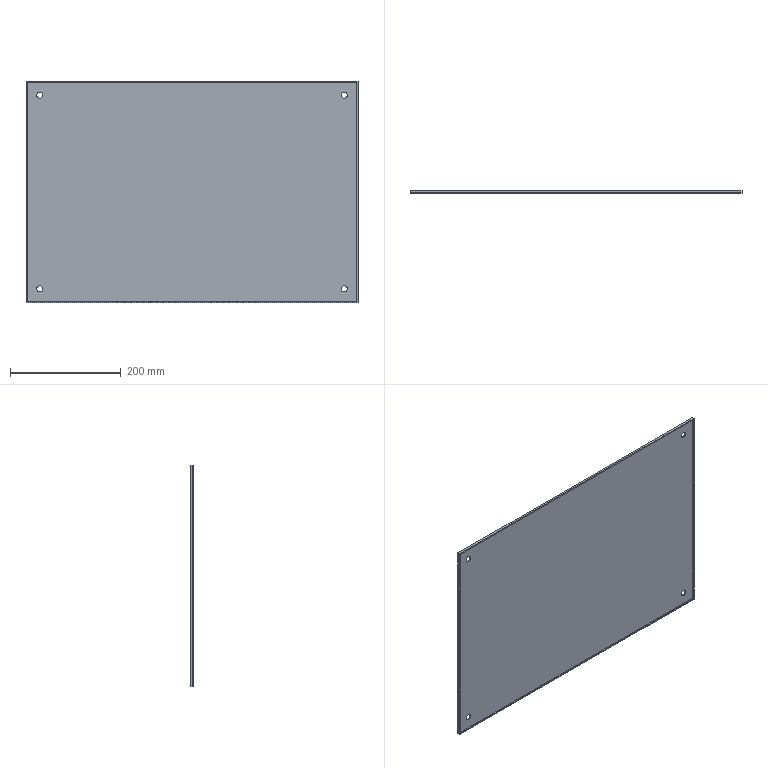Part | SolidWorks | features Cut 1, Extrusion 1, Shell 1 | 1 solid | 19 faces | box 600 x 4 x 400 mm | volume 487208 mm3 | plane 11 | cylinder 8 | commonest cylinder face diameters 11 x8
STEP:
#1=CARTESIAN_POINT('',(-275.,2.,169.5));
#2=VERTEX_POINT('',#1);
#3=CARTESIAN_POINT('',(-275.,2.,180.5));
#4=VERTEX_POINT('',#3);
#5=CARTESIAN_POINT('',(-275.,2.,175.));
#6=DIRECTION('',(0.,1.,0.));
#7=DIRECTION('',(0.,0.,1.));
#8=AXIS2_PLACEMENT_3D('',#5,#6,#7);
#9=CIRCLE('',#8,5.5);
#10=EDGE_CURVE('',#2,#4,#9,.T.);
#11=ORIENTED_EDGE('',*,*,#10,.F.);
#12=CARTESIAN_POINT('',(-275.,4.,169.5));
#13=VERTEX_POINT('',#12);
#14=CARTESIAN_POINT('',(-275.,0.,169.5));
#15=DIRECTION('',(0.,1.,0.));
#16=VECTOR('',#15,1000.);
#17=LINE('',#14,#16);
#18=EDGE_CURVE('',#2,#13,#17,.T.);
#19=ORIENTED_EDGE('',*,*,#18,.T.);
#20=CARTESIAN_POINT('',(-275.,4.,180.5));
#21=VERTEX_POINT('',#20);
#22=CARTESIAN_POINT('',(-275.,4.,175.));
#23=DIRECTION('',(0.,1.,0.));
#24=DIRECTION('',(0.,0.,1.));
#25=AXIS2_PLACEMENT_3D('',#22,#23,#24);
#26=CIRCLE('',#25,5.5);
#27=EDGE_CURVE('',#13,#21,#26,.T.);
#28=ORIENTED_EDGE('',*,*,#27,.T.);
#29=CARTESIAN_POINT('',(-275.,0.,180.5));
#30=DIRECTION('',(0.,1.,0.));
#31=VECTOR('',#30,1000.);
#32=LINE('',#29,#31);
#33=EDGE_CURVE('',#4,#21,#32,.T.);
#34=ORIENTED_EDGE('',*,*,#33,.F.);
#35=EDGE_LOOP('',(#11,#19,#28,#34));
#36=FACE_OUTER_BOUND('',#35,.T.);
#37=CARTESIAN_POINT('',(-275.,0.,175.));
#38=DIRECTION('',(0.,1.,0.));
#39=DIRECTION('',(0.,0.,1.));
#40=AXIS2_PLACEMENT_3D('',#37,#38,#39);
#41=CYLINDRICAL_SURFACE('',#40,5.5);
#42=ADVANCED_FACE('',(#36),#41,.F.);
#43=CARTESIAN_POINT('',(275.,2.,169.5));
#44=VERTEX_POINT('',#43);
#45=CARTESIAN_POINT('',(275.,2.,180.5));
#46=VERTEX_POINT('',#45);
#47=CARTESIAN_POINT('',(275.,2.,175.));
#48=DIRECTION('',(0.,1.,0.));
#49=DIRECTION('',(0.,0.,1.));
#50=AXIS2_PLACEMENT_3D('',#47,#48,#49);
#51=CIRCLE('',#50,5.5);
#52=EDGE_CURVE('',#44,#46,#51,.T.);
#53=ORIENTED_EDGE('',*,*,#52,.F.);
#54=CARTESIAN_POINT('',(275.,4.,169.5));
#55=VERTEX_POINT('',#54);
#56=CARTESIAN_POINT('',(275.,0.,169.5));
#57=DIRECTION('',(0.,1.,0.));
#58=VECTOR('',#57,1000.);
#59=LINE('',#56,#58);
#60=EDGE_CURVE('',#44,#55,#59,.T.);
#61=ORIENTED_EDGE('',*,*,#60,.T.);
#62=CARTESIAN_POINT('',(275.,4.,180.5));
#63=VERTEX_POINT('',#62);
#64=CARTESIAN_POINT('',(275.,4.,175.));
#65=DIRECTION('',(0.,1.,0.));
#66=DIRECTION('',(0.,0.,1.));
#67=AXIS2_PLACEMENT_3D('',#64,#65,#66);
#68=CIRCLE('',#67,5.5);
#69=EDGE_CURVE('',#55,#63,#68,.T.);
#70=ORIENTED_EDGE('',*,*,#69,.T.);
#71=CARTESIAN_POINT('',(275.,0.,180.5));
#72=DIRECTION('',(0.,1.,0.));
#73=VECTOR('',#72,1000.);
#74=LINE('',#71,#73);
#75=EDGE_CURVE('',#46,#63,#74,.T.);
#76=ORIENTED_EDGE('',*,*,#75,.F.);
#77=EDGE_LOOP('',(#53,#61,#70,#76));
#78=FACE_OUTER_BOUND('',#77,.T.);
#79=CARTESIAN_POINT('',(275.,0.,175.));
#80=DIRECTION('',(0.,1.,0.));
#81=DIRECTION('',(0.,0.,1.));
#82=AXIS2_PLACEMENT_3D('',#79,#80,#81);
#83=CYLINDRICAL_SURFACE('',#82,5.5);
#84=ADVANCED_FACE('',(#78),#83,.F.);
#85=CARTESIAN_POINT('',(275.,2.,-180.5));
#86=VERTEX_POINT('',#85);
#87=CARTESIAN_POINT('',(275.,2.,-169.5));
#88=VERTEX_POINT('',#87);
#89=CARTESIAN_POINT('',(275.,2.,-175.));
#90=DIRECTION('',(0.,1.,0.));
#91=DIRECTION('',(0.,0.,1.));
#92=AXIS2_PLACEMENT_3D('',#89,#90,#91);
#93=CIRCLE('',#92,5.5);
#94=EDGE_CURVE('',#86,#88,#93,.T.);
#95=ORIENTED_EDGE('',*,*,#94,.F.);
#96=CARTESIAN_POINT('',(275.,4.,-180.5));
#97=VERTEX_POINT('',#96);
#98=CARTESIAN_POINT('',(275.,0.,-180.5));
#99=DIRECTION('',(0.,1.,0.));
#100=VECTOR('',#99,1000.);
#101=LINE('',#98,#100);
#102=EDGE_CURVE('',#86,#97,#101,.T.);
#103=ORIENTED_EDGE('',*,*,#102,.T.);
#104=CARTESIAN_POINT('',(275.,4.,-169.5));
#105=VERTEX_POINT('',#104);
#106=CARTESIAN_POINT('',(275.,4.,-175.));
#107=DIRECTION('',(0.,1.,0.));
#108=DIRECTION('',(0.,0.,1.));
#109=AXIS2_PLACEMENT_3D('',#106,#107,#108);
#110=CIRCLE('',#109,5.5);
#111=EDGE_CURVE('',#97,#105,#110,.T.);
#112=ORIENTED_EDGE('',*,*,#111,.T.);
#113=CARTESIAN_POINT('',(275.,0.,-169.5));
#114=DIRECTION('',(0.,1.,0.));
#115=VECTOR('',#114,1000.);
#116=LINE('',#113,#115);
#117=EDGE_CURVE('',#88,#105,#116,.T.);
#118=ORIENTED_EDGE('',*,*,#117,.F.);
#119=EDGE_LOOP('',(#95,#103,#112,#118));
#120=FACE_OUTER_BOUND('',#119,.T.);
#121=CARTESIAN_POINT('',(275.,0.,-175.));
#122=DIRECTION('',(0.,1.,0.));
#123=DIRECTION('',(0.,0.,1.));
#124=AXIS2_PLACEMENT_3D('',#121,#122,#123);
#125=CYLINDRICAL_SURFACE('',#124,5.5);
#126=ADVANCED_FACE('',(#120),#125,.F.);
#127=CARTESIAN_POINT('',(-275.,2.,-180.5));
#128=VERTEX_POINT('',#127);
#129=CARTESIAN_POINT('',(-275.,2.,-169.5));
#130=VERTEX_POINT('',#129);
#131=CARTESIAN_POINT('',(-275.,2.,-175.));
#132=DIRECTION('',(0.,1.,0.));
#133=DIRECTION('',(0.,0.,1.));
#134=AXIS2_PLACEMENT_3D('',#131,#132,#133);
#135=CIRCLE('',#134,5.5);
#136=EDGE_CURVE('',#128,#130,#135,.T.);
#137=ORIENTED_EDGE('',*,*,#136,.F.);
#138=CARTESIAN_POINT('',(-275.,4.,-180.5));
#139=VERTEX_POINT('',#138);
#140=CARTESIAN_POINT('',(-275.,0.,-180.5));
#141=DIRECTION('',(0.,1.,0.));
#142=VECTOR('',#141,1000.);
#143=LINE('',#140,#142);
#144=EDGE_CURVE('',#128,#139,#143,.T.);
#145=ORIENTED_EDGE('',*,*,#144,.T.);
#146=CARTESIAN_POINT('',(-275.,4.,-169.5));
#147=VERTEX_POINT('',#146);
#148=CARTESIAN_POINT('',(-275.,4.,-175.));
#149=DIRECTION('',(0.,1.,0.));
#150=DIRECTION('',(0.,0.,1.));
#151=AXIS2_PLACEMENT_3D('',#148,#149,#150);
#152=CIRCLE('',#151,5.5);
#153=EDGE_CURVE('',#139,#147,#152,.T.);
#154=ORIENTED_EDGE('',*,*,#153,.T.);
#155=CARTESIAN_POINT('',(-275.,0.,-169.5));
#156=DIRECTION('',(0.,1.,0.));
#157=VECTOR('',#156,1000.);
#158=LINE('',#155,#157);
#159=EDGE_CURVE('',#130,#147,#158,.T.);
#160=ORIENTED_EDGE('',*,*,#159,.F.);
#161=EDGE_LOOP('',(#137,#145,#154,#160));
#162=FACE_OUTER_BOUND('',#161,.T.);
#163=CARTESIAN_POINT('',(-275.,0.,-175.));
#164=DIRECTION('',(0.,1.,0.));
#165=DIRECTION('',(0.,0.,1.));
#166=AXIS2_PLACEMENT_3D('',#163,#164,#165);
#167=CYLINDRICAL_SURFACE('',#166,5.5);
#168=ADVANCED_FACE('',(#162),#167,.F.);
#169=CARTESIAN_POINT('',(300.,0.,200.));
#170=VERTEX_POINT('',#169);
#171=CARTESIAN_POINT('',(300.,0.,-200.));
#172=VERTEX_POINT('',#171);
#173=CARTESIAN_POINT('',(300.,0.,-200.));
#174=DIRECTION('',(0.,0.,-1.));
#175=VECTOR('',#174,1000.);
#176=LINE('',#173,#175);
#177=EDGE_CURVE('',#170,#172,#176,.T.);
#178=ORIENTED_EDGE('',*,*,#177,.T.);
#179=CARTESIAN_POINT('',(300.,4.,-200.));
#180=VERTEX_POINT('',#179);
#181=CARTESIAN_POINT('',(300.,4.,-200.));
#182=DIRECTION('',(0.,-1.,0.));
#183=VECTOR('',#182,1000.);
#184=LINE('',#181,#183);
#185=EDGE_CURVE('',#180,#172,#184,.T.);
#186=ORIENTED_EDGE('',*,*,#185,.F.);
#187=CARTESIAN_POINT('',(300.,4.,200.));
#188=VERTEX_POINT('',#187);
#189=CARTESIAN_POINT('',(300.,4.,-200.));
#190=DIRECTION('',(0.,0.,-1.));
#191=VECTOR('',#190,1000.);
#192=LINE('',#189,#191);
#193=EDGE_CURVE('',#188,#180,#192,.T.);
#194=ORIENTED_EDGE('',*,*,#193,.F.);
#195=CARTESIAN_POINT('',(300.,4.,200.));
#196=DIRECTION('',(0.,-1.,0.));
#197=VECTOR('',#196,1000.);
#198=LINE('',#195,#197);
#199=EDGE_CURVE('',#188,#170,#198,.T.);
#200=ORIENTED_EDGE('',*,*,#199,.T.);
#201=EDGE_LOOP('',(#178,#186,#194,#200));
#202=FACE_OUTER_BOUND('',#201,.T.);
#203=CARTESIAN_POINT('',(300.,4.,-200.));
#204=DIRECTION('',(-1.,0.,0.));
#205=DIRECTION('',(0.,0.,1.));
#206=AXIS2_PLACEMENT_3D('',#203,#204,#205);
#207=PLANE('',#206);
#208=ADVANCED_FACE('',(#202),#207,.F.);
#209=CARTESIAN_POINT('',(-300.,0.,-200.));
#210=VERTEX_POINT('',#209);
#211=CARTESIAN_POINT('',(-300.,0.,-200.));
#212=DIRECTION('',(-1.,0.,0.));
#213=VECTOR('',#212,1000.);
#214=LINE('',#211,#213);
#215=EDGE_CURVE('',#172,#210,#214,.T.);
#216=ORIENTED_EDGE('',*,*,#215,.T.);
#217=CARTESIAN_POINT('',(-300.,4.,-200.));
#218=VERTEX_POINT('',#217);
#219=CARTESIAN_POINT('',(-300.,4.,-200.));
#220=DIRECTION('',(0.,-1.,0.));
#221=VECTOR('',#220,1000.);
#222=LINE('',#219,#221);
#223=EDGE_CURVE('',#218,#210,#222,.T.);
#224=ORIENTED_EDGE('',*,*,#223,.F.);
#225=CARTESIAN_POINT('',(-300.,4.,-200.));
#226=DIRECTION('',(-1.,0.,0.));
#227=VECTOR('',#226,1000.);
#228=LINE('',#225,#227);
#229=EDGE_CURVE('',#180,#218,#228,.T.);
#230=ORIENTED_EDGE('',*,*,#229,.F.);
#231=ORIENTED_EDGE('',*,*,#185,.T.);
#232=EDGE_LOOP('',(#216,#224,#230,#231));
#233=FACE_OUTER_BOUND('',#232,.T.);
#234=CARTESIAN_POINT('',(-300.,4.,-200.));
#235=DIRECTION('',(0.,0.,1.));
#236=DIRECTION('',(1.,0.,0.));
#237=AXIS2_PLACEMENT_3D('',#234,#235,#236);
#238=PLANE('',#237);
#239=ADVANCED_FACE('',(#233),#238,.F.);
#240=CARTESIAN_POINT('',(-300.,0.,200.));
#241=VERTEX_POINT('',#240);
#242=CARTESIAN_POINT('',(-300.,0.,-200.));
#243=DIRECTION('',(0.,0.,1.));
#244=VECTOR('',#243,1000.);
#245=LINE('',#242,#244);
#246=EDGE_CURVE('',#210,#241,#245,.T.);
#247=ORIENTED_EDGE('',*,*,#246,.T.);
#248=CARTESIAN_POINT('',(-300.,4.,200.));
#249=VERTEX_POINT('',#248);
#250=CARTESIAN_POINT('',(-300.,4.,200.));
#251=DIRECTION('',(0.,-1.,0.));
#252=VECTOR('',#251,1000.);
#253=LINE('',#250,#252);
#254=EDGE_CURVE('',#249,#241,#253,.T.);
#255=ORIENTED_EDGE('',*,*,#254,.F.);
#256=CARTESIAN_POINT('',(-300.,4.,-200.));
#257=DIRECTION('',(0.,0.,1.));
#258=VECTOR('',#257,1000.);
#259=LINE('',#256,#258);
#260=EDGE_CURVE('',#218,#249,#259,.T.);
#261=ORIENTED_EDGE('',*,*,#260,.F.);
#262=ORIENTED_EDGE('',*,*,#223,.T.);
#263=EDGE_LOOP('',(#247,#255,#261,#262));
#264=FACE_OUTER_BOUND('',#263,.T.);
#265=CARTESIAN_POINT('',(-300.,4.,-200.));
#266=DIRECTION('',(1.,0.,0.));
#267=DIRECTION('',(0.,0.,-1.));
#268=AXIS2_PLACEMENT_3D('',#265,#266,#267);
#269=PLANE('',#268);
#270=ADVANCED_FACE('',(#264),#269,.F.);
#271=CARTESIAN_POINT('',(-300.,0.,200.));
#272=DIRECTION('',(1.,0.,0.));
#273=VECTOR('',#272,1000.);
#274=LINE('',#271,#273);
#275=EDGE_CURVE('',#241,#170,#274,.T.);
#276=ORIENTED_EDGE('',*,*,#275,.T.);
#277=ORIENTED_EDGE('',*,*,#199,.F.);
#278=CARTESIAN_POINT('',(-300.,4.,200.));
#279=DIRECTION('',(1.,0.,0.));
#280=VECTOR('',#279,1000.);
#281=LINE('',#278,#280);
#282=EDGE_CURVE('',#249,#188,#281,.T.);
#283=ORIENTED_EDGE('',*,*,#282,.F.);
#284=ORIENTED_EDGE('',*,*,#254,.T.);
#285=EDGE_LOOP('',(#276,#277,#283,#284));
#286=FACE_OUTER_BOUND('',#285,.T.);
#287=CARTESIAN_POINT('',(-300.,4.,200.));
#288=DIRECTION('',(0.,0.,-1.));
#289=DIRECTION('',(-1.,0.,0.));
#290=AXIS2_PLACEMENT_3D('',#287,#288,#289);
#291=PLANE('',#290);
#292=ADVANCED_FACE('',(#286),#291,.F.);
#293=CARTESIAN_POINT('',(-275.,4.,175.));
#294=DIRECTION('',(0.,1.,0.));
#295=DIRECTION('',(0.,0.,1.));
#296=AXIS2_PLACEMENT_3D('',#293,#294,#295);
#297=CIRCLE('',#296,5.5);
#298=EDGE_CURVE('',#21,#13,#297,.T.);
#299=ORIENTED_EDGE('',*,*,#298,.F.);
#300=ORIENTED_EDGE('',*,*,#27,.F.);
#301=EDGE_LOOP('',(#299,#300));
#302=FACE_BOUND('',#301,.T.);
#303=CARTESIAN_POINT('',(275.,4.,175.));
#304=DIRECTION('',(0.,1.,0.));
#305=DIRECTION('',(0.,0.,1.));
#306=AXIS2_PLACEMENT_3D('',#303,#304,#305);
#307=CIRCLE('',#306,5.5);
#308=EDGE_CURVE('',#63,#55,#307,.T.);
#309=ORIENTED_EDGE('',*,*,#308,.F.);
#310=ORIENTED_EDGE('',*,*,#69,.F.);
#311=EDGE_LOOP('',(#309,#310));
#312=FACE_BOUND('',#311,.T.);
#313=CARTESIAN_POINT('',(275.,4.,-175.));
#314=DIRECTION('',(0.,1.,0.));
#315=DIRECTION('',(0.,0.,1.));
#316=AXIS2_PLACEMENT_3D('',#313,#314,#315);
#317=CIRCLE('',#316,5.5);
#318=EDGE_CURVE('',#105,#97,#317,.T.);
#319=ORIENTED_EDGE('',*,*,#318,.F.);
#320=ORIENTED_EDGE('',*,*,#111,.F.);
#321=EDGE_LOOP('',(#319,#320));
#322=FACE_BOUND('',#321,.T.);
#323=CARTESIAN_POINT('',(-275.,4.,-175.));
#324=DIRECTION('',(0.,1.,0.));
#325=DIRECTION('',(0.,0.,1.));
#326=AXIS2_PLACEMENT_3D('',#323,#324,#325);
#327=CIRCLE('',#326,5.5);
#328=EDGE_CURVE('',#147,#139,#327,.T.);
#329=ORIENTED_EDGE('',*,*,#328,.F.);
#330=ORIENTED_EDGE('',*,*,#153,.F.);
#331=EDGE_LOOP('',(#329,#330));
#332=FACE_BOUND('',#331,.T.);
#333=ORIENTED_EDGE('',*,*,#193,.T.);
#334=ORIENTED_EDGE('',*,*,#229,.T.);
#335=ORIENTED_EDGE('',*,*,#260,.T.);
#336=ORIENTED_EDGE('',*,*,#282,.T.);
#337=EDGE_LOOP('',(#333,#334,#335,#336));
#338=FACE_OUTER_BOUND('',#337,.T.);
#339=CARTESIAN_POINT('',(0.,4.,0.));
#340=DIRECTION('',(0.,1.,0.));
#341=DIRECTION('',(0.,0.,1.));
#342=AXIS2_PLACEMENT_3D('',#339,#340,#341);
#343=PLANE('',#342);
#344=ADVANCED_FACE('',(#302,#312,#322,#332,#338),#343,.T.);
#345=CARTESIAN_POINT('',(-298.,0.,198.));
#346=VERTEX_POINT('',#345);
#347=CARTESIAN_POINT('',(298.,0.,198.));
#348=VERTEX_POINT('',#347);
#349=CARTESIAN_POINT('',(-300.,0.,198.));
#350=DIRECTION('',(1.,0.,0.));
#351=VECTOR('',#350,1000.);
#352=LINE('',#349,#351);
#353=EDGE_CURVE('',#346,#348,#352,.T.);
#354=ORIENTED_EDGE('',*,*,#353,.T.);
#355=CARTESIAN_POINT('',(298.,0.,-198.));
#356=VERTEX_POINT('',#355);
#357=CARTESIAN_POINT('',(298.,0.,-200.));
#358=DIRECTION('',(0.,0.,-1.));
#359=VECTOR('',#358,1000.);
#360=LINE('',#357,#359);
#361=EDGE_CURVE('',#348,#356,#360,.T.);
#362=ORIENTED_EDGE('',*,*,#361,.T.);
#363=CARTESIAN_POINT('',(-298.,0.,-198.));
#364=VERTEX_POINT('',#363);
#365=CARTESIAN_POINT('',(-300.,0.,-198.));
#366=DIRECTION('',(-1.,0.,0.));
#367=VECTOR('',#366,1000.);
#368=LINE('',#365,#367);
#369=EDGE_CURVE('',#356,#364,#368,.T.);
#370=ORIENTED_EDGE('',*,*,#369,.T.);
#371=CARTESIAN_POINT('',(-298.,0.,-200.));
#372=DIRECTION('',(0.,0.,1.));
#373=VECTOR('',#372,1000.);
#374=LINE('',#371,#373);
#375=EDGE_CURVE('',#364,#346,#374,.T.);
#376=ORIENTED_EDGE('',*,*,#375,.T.);
#377=EDGE_LOOP('',(#354,#362,#370,#376));
#378=FACE_BOUND('',#377,.T.);
#379=ORIENTED_EDGE('',*,*,#177,.F.);
#380=ORIENTED_EDGE('',*,*,#275,.F.);
#381=ORIENTED_EDGE('',*,*,#246,.F.);
#382=ORIENTED_EDGE('',*,*,#215,.F.);
#383=EDGE_LOOP('',(#379,#380,#381,#382));
#384=FACE_OUTER_BOUND('',#383,.T.);
#385=CARTESIAN_POINT('',(0.,0.,0.));
#386=DIRECTION('',(0.,1.,0.));
#387=DIRECTION('',(0.,0.,1.));
#388=AXIS2_PLACEMENT_3D('',#385,#386,#387);
#389=PLANE('',#388);
#390=ADVANCED_FACE('',(#378,#384),#389,.F.);
#391=ORIENTED_EDGE('',*,*,#361,.F.);
#392=CARTESIAN_POINT('',(298.,2.,198.));
#393=VERTEX_POINT('',#392);
#394=CARTESIAN_POINT('',(298.,4.,198.));
#395=DIRECTION('',(0.,-1.,0.));
#396=VECTOR('',#395,1000.);
#397=LINE('',#394,#396);
#398=EDGE_CURVE('',#393,#348,#397,.T.);
#399=ORIENTED_EDGE('',*,*,#398,.F.);
#400=CARTESIAN_POINT('',(298.,2.,-198.));
#401=VERTEX_POINT('',#400);
#402=CARTESIAN_POINT('',(298.,2.,-200.));
#403=DIRECTION('',(0.,0.,-1.));
#404=VECTOR('',#403,1000.);
#405=LINE('',#402,#404);
#406=EDGE_CURVE('',#393,#401,#405,.T.);
#407=ORIENTED_EDGE('',*,*,#406,.T.);
#408=CARTESIAN_POINT('',(298.,4.,-198.));
#409=DIRECTION('',(0.,-1.,0.));
#410=VECTOR('',#409,1000.);
#411=LINE('',#408,#410);
#412=EDGE_CURVE('',#401,#356,#411,.T.);
#413=ORIENTED_EDGE('',*,*,#412,.T.);
#414=EDGE_LOOP('',(#391,#399,#407,#413));
#415=FACE_OUTER_BOUND('',#414,.T.);
#416=CARTESIAN_POINT('',(298.,4.,-200.));
#417=DIRECTION('',(-1.,0.,0.));
#418=DIRECTION('',(0.,0.,1.));
#419=AXIS2_PLACEMENT_3D('',#416,#417,#418);
#420=PLANE('',#419);
#421=ADVANCED_FACE('',(#415),#420,.T.);
#422=ORIENTED_EDGE('',*,*,#369,.F.);
#423=ORIENTED_EDGE('',*,*,#412,.F.);
#424=CARTESIAN_POINT('',(-298.,2.,-198.));
#425=VERTEX_POINT('',#424);
#426=CARTESIAN_POINT('',(-300.,2.,-198.));
#427=DIRECTION('',(-1.,0.,0.));
#428=VECTOR('',#427,1000.);
#429=LINE('',#426,#428);
#430=EDGE_CURVE('',#401,#425,#429,.T.);
#431=ORIENTED_EDGE('',*,*,#430,.T.);
#432=CARTESIAN_POINT('',(-298.,4.,-198.));
#433=DIRECTION('',(0.,-1.,0.));
#434=VECTOR('',#433,1000.);
#435=LINE('',#432,#434);
#436=EDGE_CURVE('',#425,#364,#435,.T.);
#437=ORIENTED_EDGE('',*,*,#436,.T.);
#438=EDGE_LOOP('',(#422,#423,#431,#437));
#439=FACE_OUTER_BOUND('',#438,.T.);
#440=CARTESIAN_POINT('',(-300.,4.,-198.));
#441=DIRECTION('',(0.,0.,1.));
#442=DIRECTION('',(1.,0.,0.));
#443=AXIS2_PLACEMENT_3D('',#440,#441,#442);
#444=PLANE('',#443);
#445=ADVANCED_FACE('',(#439),#444,.T.);
#446=ORIENTED_EDGE('',*,*,#375,.F.);
#447=ORIENTED_EDGE('',*,*,#436,.F.);
#448=CARTESIAN_POINT('',(-298.,2.,198.));
#449=VERTEX_POINT('',#448);
#450=CARTESIAN_POINT('',(-298.,2.,-200.));
#451=DIRECTION('',(0.,0.,1.));
#452=VECTOR('',#451,1000.);
#453=LINE('',#450,#452);
#454=EDGE_CURVE('',#425,#449,#453,.T.);
#455=ORIENTED_EDGE('',*,*,#454,.T.);
#456=CARTESIAN_POINT('',(-298.,4.,198.));
#457=DIRECTION('',(0.,-1.,0.));
#458=VECTOR('',#457,1000.);
#459=LINE('',#456,#458);
#460=EDGE_CURVE('',#449,#346,#459,.T.);
#461=ORIENTED_EDGE('',*,*,#460,.T.);
#462=EDGE_LOOP('',(#446,#447,#455,#461));
#463=FACE_OUTER_BOUND('',#462,.T.);
#464=CARTESIAN_POINT('',(-298.,4.,-200.));
#465=DIRECTION('',(1.,0.,0.));
#466=DIRECTION('',(0.,0.,-1.));
#467=AXIS2_PLACEMENT_3D('',#464,#465,#466);
#468=PLANE('',#467);
#469=ADVANCED_FACE('',(#463),#468,.T.);
#470=ORIENTED_EDGE('',*,*,#353,.F.);
#471=ORIENTED_EDGE('',*,*,#460,.F.);
#472=CARTESIAN_POINT('',(-300.,2.,198.));
#473=DIRECTION('',(1.,0.,0.));
#474=VECTOR('',#473,1000.);
#475=LINE('',#472,#474);
#476=EDGE_CURVE('',#449,#393,#475,.T.);
#477=ORIENTED_EDGE('',*,*,#476,.T.);
#478=ORIENTED_EDGE('',*,*,#398,.T.);
#479=EDGE_LOOP('',(#470,#471,#477,#478));
#480=FACE_OUTER_BOUND('',#479,.T.);
#481=CARTESIAN_POINT('',(-300.,4.,198.));
#482=DIRECTION('',(0.,0.,-1.));
#483=DIRECTION('',(-1.,0.,0.));
#484=AXIS2_PLACEMENT_3D('',#481,#482,#483);
#485=PLANE('',#484);
#486=ADVANCED_FACE('',(#480),#485,.T.);
#487=CARTESIAN_POINT('',(-275.,2.,175.));
#488=DIRECTION('',(0.,1.,0.));
#489=DIRECTION('',(0.,0.,1.));
#490=AXIS2_PLACEMENT_3D('',#487,#488,#489);
#491=CIRCLE('',#490,5.5);
#492=EDGE_CURVE('',#4,#2,#491,.T.);
#493=ORIENTED_EDGE('',*,*,#492,.T.);
#494=ORIENTED_EDGE('',*,*,#10,.T.);
#495=EDGE_LOOP('',(#493,#494));
#496=FACE_BOUND('',#495,.T.);
#497=CARTESIAN_POINT('',(275.,2.,175.));
#498=DIRECTION('',(0.,1.,0.));
#499=DIRECTION('',(0.,0.,1.));
#500=AXIS2_PLACEMENT_3D('',#497,#498,#499);
#501=CIRCLE('',#500,5.5);
#502=EDGE_CURVE('',#46,#44,#501,.T.);
#503=ORIENTED_EDGE('',*,*,#502,.T.);
#504=ORIENTED_EDGE('',*,*,#52,.T.);
#505=EDGE_LOOP('',(#503,#504));
#506=FACE_BOUND('',#505,.T.);
#507=CARTESIAN_POINT('',(275.,2.,-175.));
#508=DIRECTION('',(0.,1.,0.));
#509=DIRECTION('',(0.,0.,1.));
#510=AXIS2_PLACEMENT_3D('',#507,#508,#509);
#511=CIRCLE('',#510,5.5);
#512=EDGE_CURVE('',#88,#86,#511,.T.);
#513=ORIENTED_EDGE('',*,*,#512,.T.);
#514=ORIENTED_EDGE('',*,*,#94,.T.);
#515=EDGE_LOOP('',(#513,#514));
#516=FACE_BOUND('',#515,.T.);
#517=CARTESIAN_POINT('',(-275.,2.,-175.));
#518=DIRECTION('',(0.,1.,0.));
#519=DIRECTION('',(0.,0.,1.));
#520=AXIS2_PLACEMENT_3D('',#517,#518,#519);
#521=CIRCLE('',#520,5.5);
#522=EDGE_CURVE('',#130,#128,#521,.T.);
#523=ORIENTED_EDGE('',*,*,#522,.T.);
#524=ORIENTED_EDGE('',*,*,#136,.T.);
#525=EDGE_LOOP('',(#523,#524));
#526=FACE_BOUND('',#525,.T.);
#527=ORIENTED_EDGE('',*,*,#406,.F.);
#528=ORIENTED_EDGE('',*,*,#476,.F.);
#529=ORIENTED_EDGE('',*,*,#454,.F.);
#530=ORIENTED_EDGE('',*,*,#430,.F.);
#531=EDGE_LOOP('',(#527,#528,#529,#530));
#532=FACE_OUTER_BOUND('',#531,.T.);
#533=CARTESIAN_POINT('',(0.,2.,0.));
#534=DIRECTION('',(0.,1.,0.));
#535=DIRECTION('',(0.,0.,1.));
#536=AXIS2_PLACEMENT_3D('',#533,#534,#535);
#537=PLANE('',#536);
#538=ADVANCED_FACE('',(#496,#506,#516,#526,#532),#537,.F.);
#539=ORIENTED_EDGE('',*,*,#144,.F.);
#540=ORIENTED_EDGE('',*,*,#522,.F.);
#541=ORIENTED_EDGE('',*,*,#159,.T.);
#542=ORIENTED_EDGE('',*,*,#328,.T.);
#543=EDGE_LOOP('',(#539,#540,#541,#542));
#544=FACE_OUTER_BOUND('',#543,.T.);
#545=CARTESIAN_POINT('',(-275.,0.,-175.));
#546=DIRECTION('',(0.,1.,0.));
#547=DIRECTION('',(0.,0.,1.));
#548=AXIS2_PLACEMENT_3D('',#545,#546,#547);
#549=CYLINDRICAL_SURFACE('',#548,5.5);
#550=ADVANCED_FACE('',(#544),#549,.F.);
#551=ORIENTED_EDGE('',*,*,#102,.F.);
#552=ORIENTED_EDGE('',*,*,#512,.F.);
#553=ORIENTED_EDGE('',*,*,#117,.T.);
#554=ORIENTED_EDGE('',*,*,#318,.T.);
#555=EDGE_LOOP('',(#551,#552,#553,#554));
#556=FACE_OUTER_BOUND('',#555,.T.);
#557=CARTESIAN_POINT('',(275.,0.,-175.));
#558=DIRECTION('',(0.,1.,0.));
#559=DIRECTION('',(0.,0.,1.));
#560=AXIS2_PLACEMENT_3D('',#557,#558,#559);
#561=CYLINDRICAL_SURFACE('',#560,5.5);
#562=ADVANCED_FACE('',(#556),#561,.F.);
#563=ORIENTED_EDGE('',*,*,#60,.F.);
#564=ORIENTED_EDGE('',*,*,#502,.F.);
#565=ORIENTED_EDGE('',*,*,#75,.T.);
#566=ORIENTED_EDGE('',*,*,#308,.T.);
#567=EDGE_LOOP('',(#563,#564,#565,#566));
#568=FACE_OUTER_BOUND('',#567,.T.);
#569=CARTESIAN_POINT('',(275.,0.,175.));
#570=DIRECTION('',(0.,1.,0.));
#571=DIRECTION('',(0.,0.,1.));
#572=AXIS2_PLACEMENT_3D('',#569,#570,#571);
#573=CYLINDRICAL_SURFACE('',#572,5.5);
#574=ADVANCED_FACE('',(#568),#573,.F.);
#575=ORIENTED_EDGE('',*,*,#18,.F.);
#576=ORIENTED_EDGE('',*,*,#492,.F.);
#577=ORIENTED_EDGE('',*,*,#33,.T.);
#578=ORIENTED_EDGE('',*,*,#298,.T.);
#579=EDGE_LOOP('',(#575,#576,#577,#578));
#580=FACE_OUTER_BOUND('',#579,.T.);
#581=CARTESIAN_POINT('',(-275.,0.,175.));
#582=DIRECTION('',(0.,1.,0.));
#583=DIRECTION('',(0.,0.,1.));
#584=AXIS2_PLACEMENT_3D('',#581,#582,#583);
#585=CYLINDRICAL_SURFACE('',#584,5.5);
#586=ADVANCED_FACE('',(#580),#585,.F.);
#587=CLOSED_SHELL('',(#42,#84,#126,#168,#208,#239,#270,#292,#344,#390,#421,#445,#469,#486,#538,#550,#562,#574,#586));
#588=MANIFOLD_SOLID_BREP('',#587);
#589=CARTESIAN_POINT('',(0.,0.,0.));
#590=DIRECTION('',(0.,0.,1.));
#591=DIRECTION('',(1.,0.,0.));
#592=AXIS2_PLACEMENT_3D('',#589,#590,#591);
#593=(LENGTH_UNIT()NAMED_UNIT(*)SI_UNIT(.MILLI.,.METRE.));
#594=UNCERTAINTY_MEASURE_WITH_UNIT(LENGTH_MEASURE(0.00001),#593,'','');
#595=(NAMED_UNIT(*)PLANE_ANGLE_UNIT()SI_UNIT($,.RADIAN.));
#596=(NAMED_UNIT(*)SI_UNIT($,.STERADIAN.)SOLID_ANGLE_UNIT());
#597=(GEOMETRIC_REPRESENTATION_CONTEXT(3)GLOBAL_UNCERTAINTY_ASSIGNED_CONTEXT((#594))GLOBAL_UNIT_ASSIGNED_CONTEXT((#593,#595,#596))REPRESENTATION_CONTEXT('',''));
#598=ADVANCED_BREP_SHAPE_REPRESENTATION('',(#588,#592),#597);